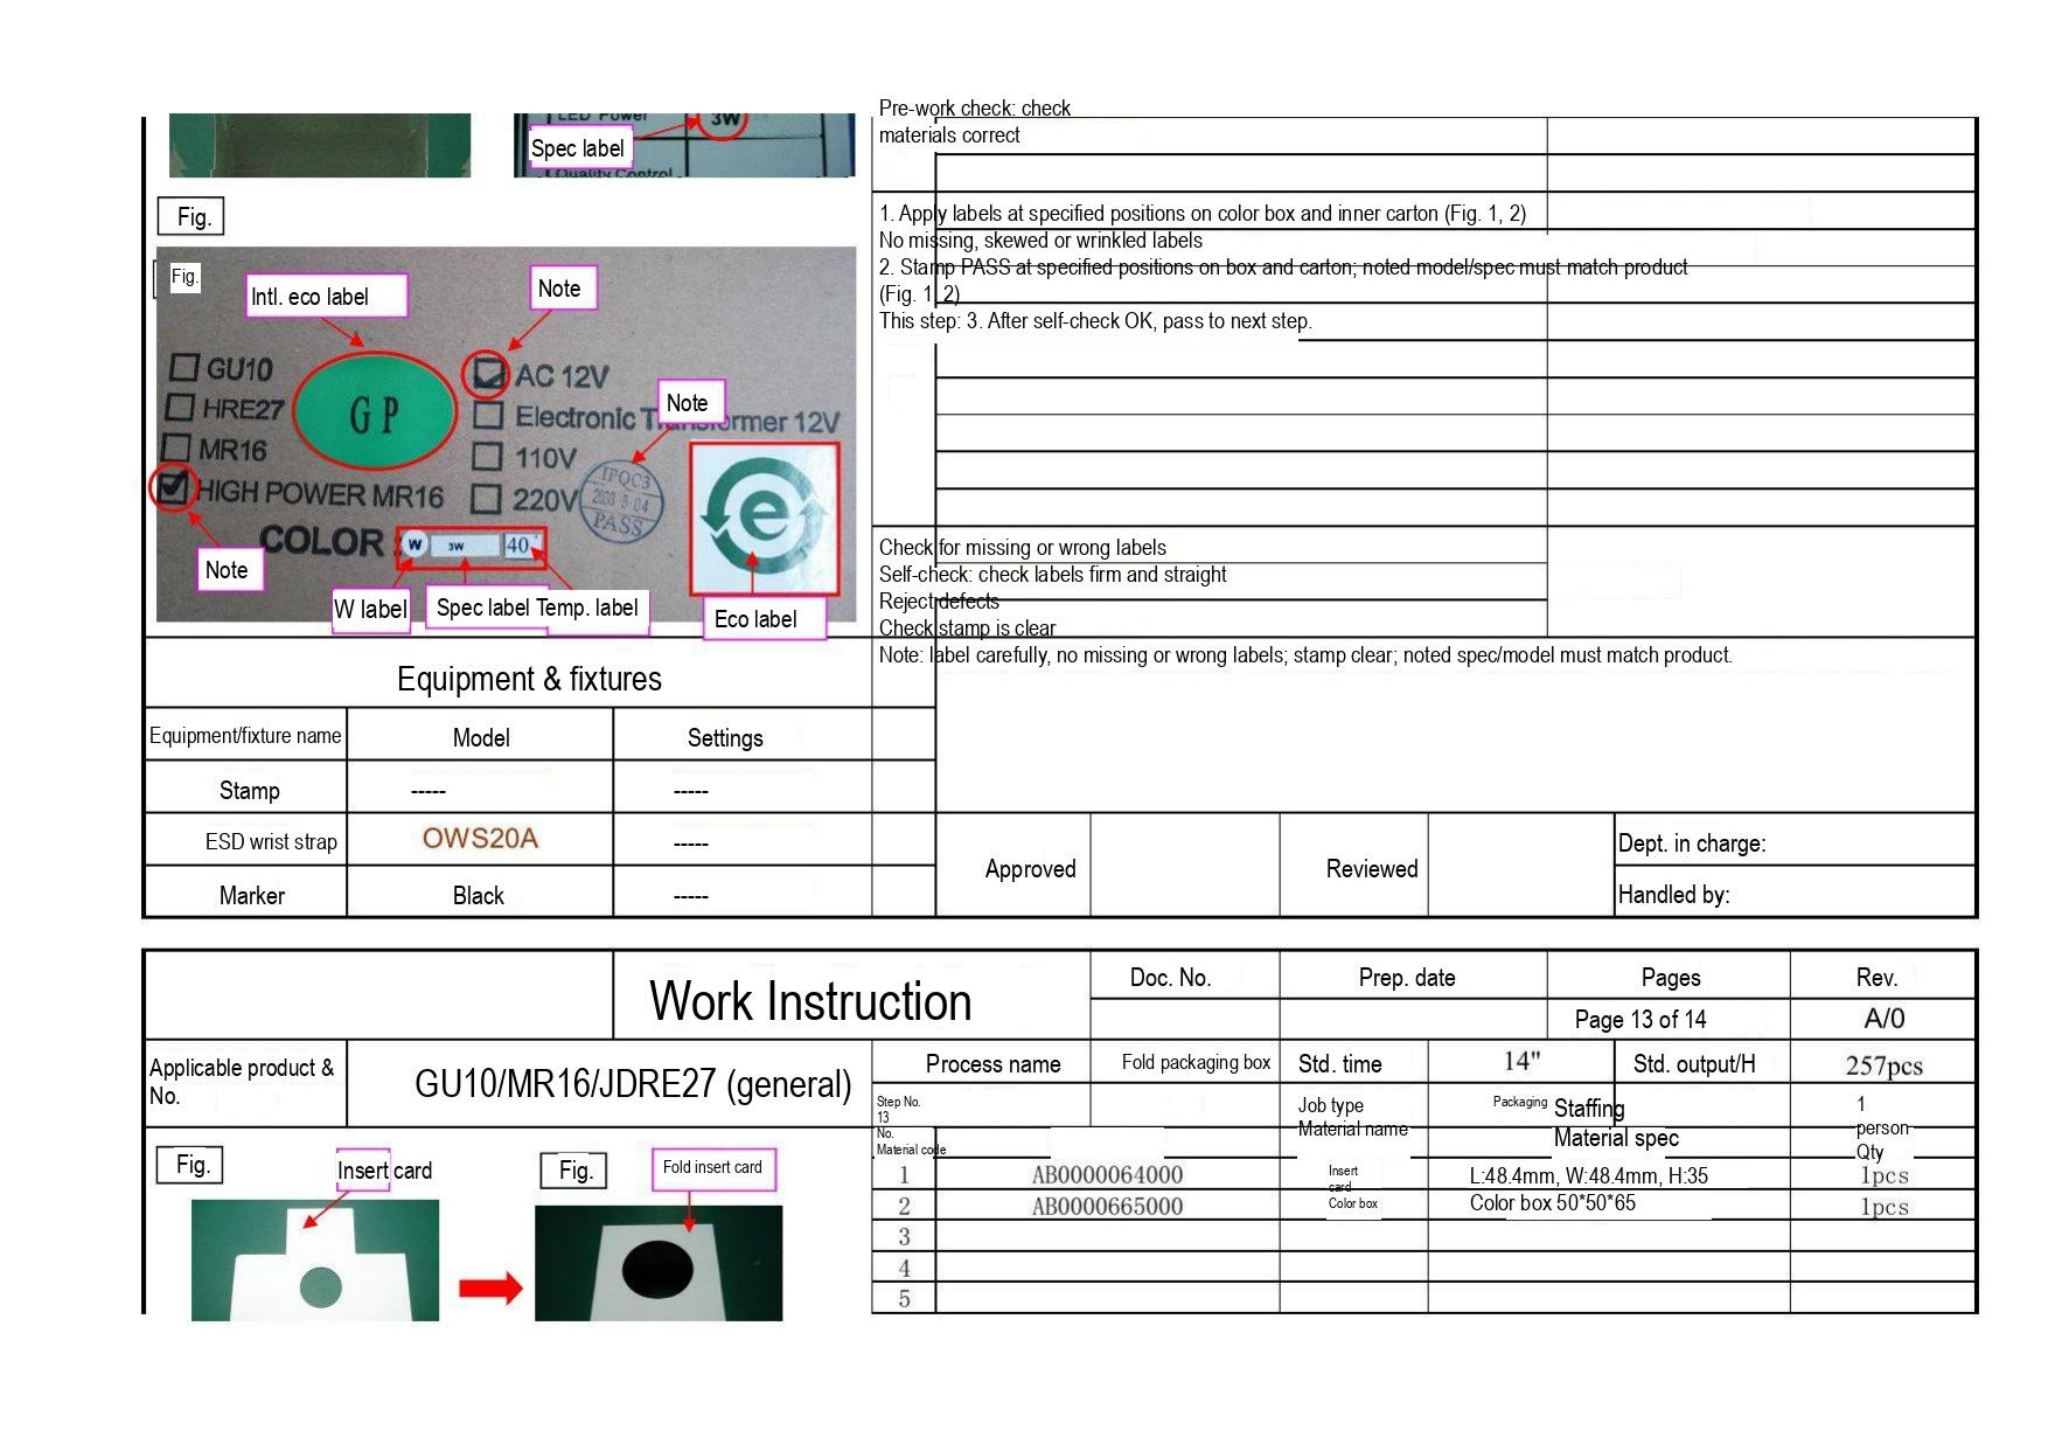LED Power

3W

Spec label

Quality Control

Fig.

Fig.

Intl. eco label

Note

GU10

HRE27

MR16

HIGH POWER MR16

G P

AC 12V

Electronic T Note rmer 12V

110V

220V

IPQC3
PASS

COLOR

W

3W

40

e

Note

W label

Spec label

Temp. label

Eco label

Pre-work check: check materials correct

1. Apply labels at specified positions on color box and inner carton (Fig. 1, 2)
No missing, skewed or wrinkled labels
2. Stamp PASS at specified positions on box and carton; noted model/spec must match product (Fig. 1, 2)
This step: 3. After self-check OK, pass to next step.

Check for missing or wrong labels
Self-check: check labels firm and straight
Reject defects
Check stamp is clear

Note: label carefully, no missing or wrong labels; stamp clear; noted spec/model must match product.

Equipment & fixtures

| Equipment/fixture name | Model | Settings |
|---|---|---|
| Stamp | ----- | ----- |
| ESD wrist strap | OWS20A | ----- |
| Marker | Black | ----- |

| Approved | | Reviewed | | Dept. in charge: |
|---|---|---|---|---|
| | | | | Handled by: |

| | Work Instruction | Doc. No. | Prep. date | Pages | Rev. |
|---|---|---|---|---|---|
| | | | | Page 13 of 14 | A/0 |

| Applicable product & No. | GU10/MR16/JDRE27 (general) |
|---|---|

| Process name | Fold packaging box | Std. time | 14" | Std. output/H | 257pcs |
|---|---|---|---|---|---|
| Step No. 13 | | Job type | Packaging | Staffing | 1 person |

| No. | Material code | Material name | Material spec | Qty |
|---|---|---|---|---|
| 1 | AB0000064000 | Insert card | L:48.4mm, W:48.4mm, H:35 | 1pcs |
| 2 | AB0000665000 | Color box | Color box 50*50*65 | 1pcs |
| 3 | | | | |
| 4 | | | | |
| 5 | | | | |

Fig.

Insert card

Fig.

Fold insert card
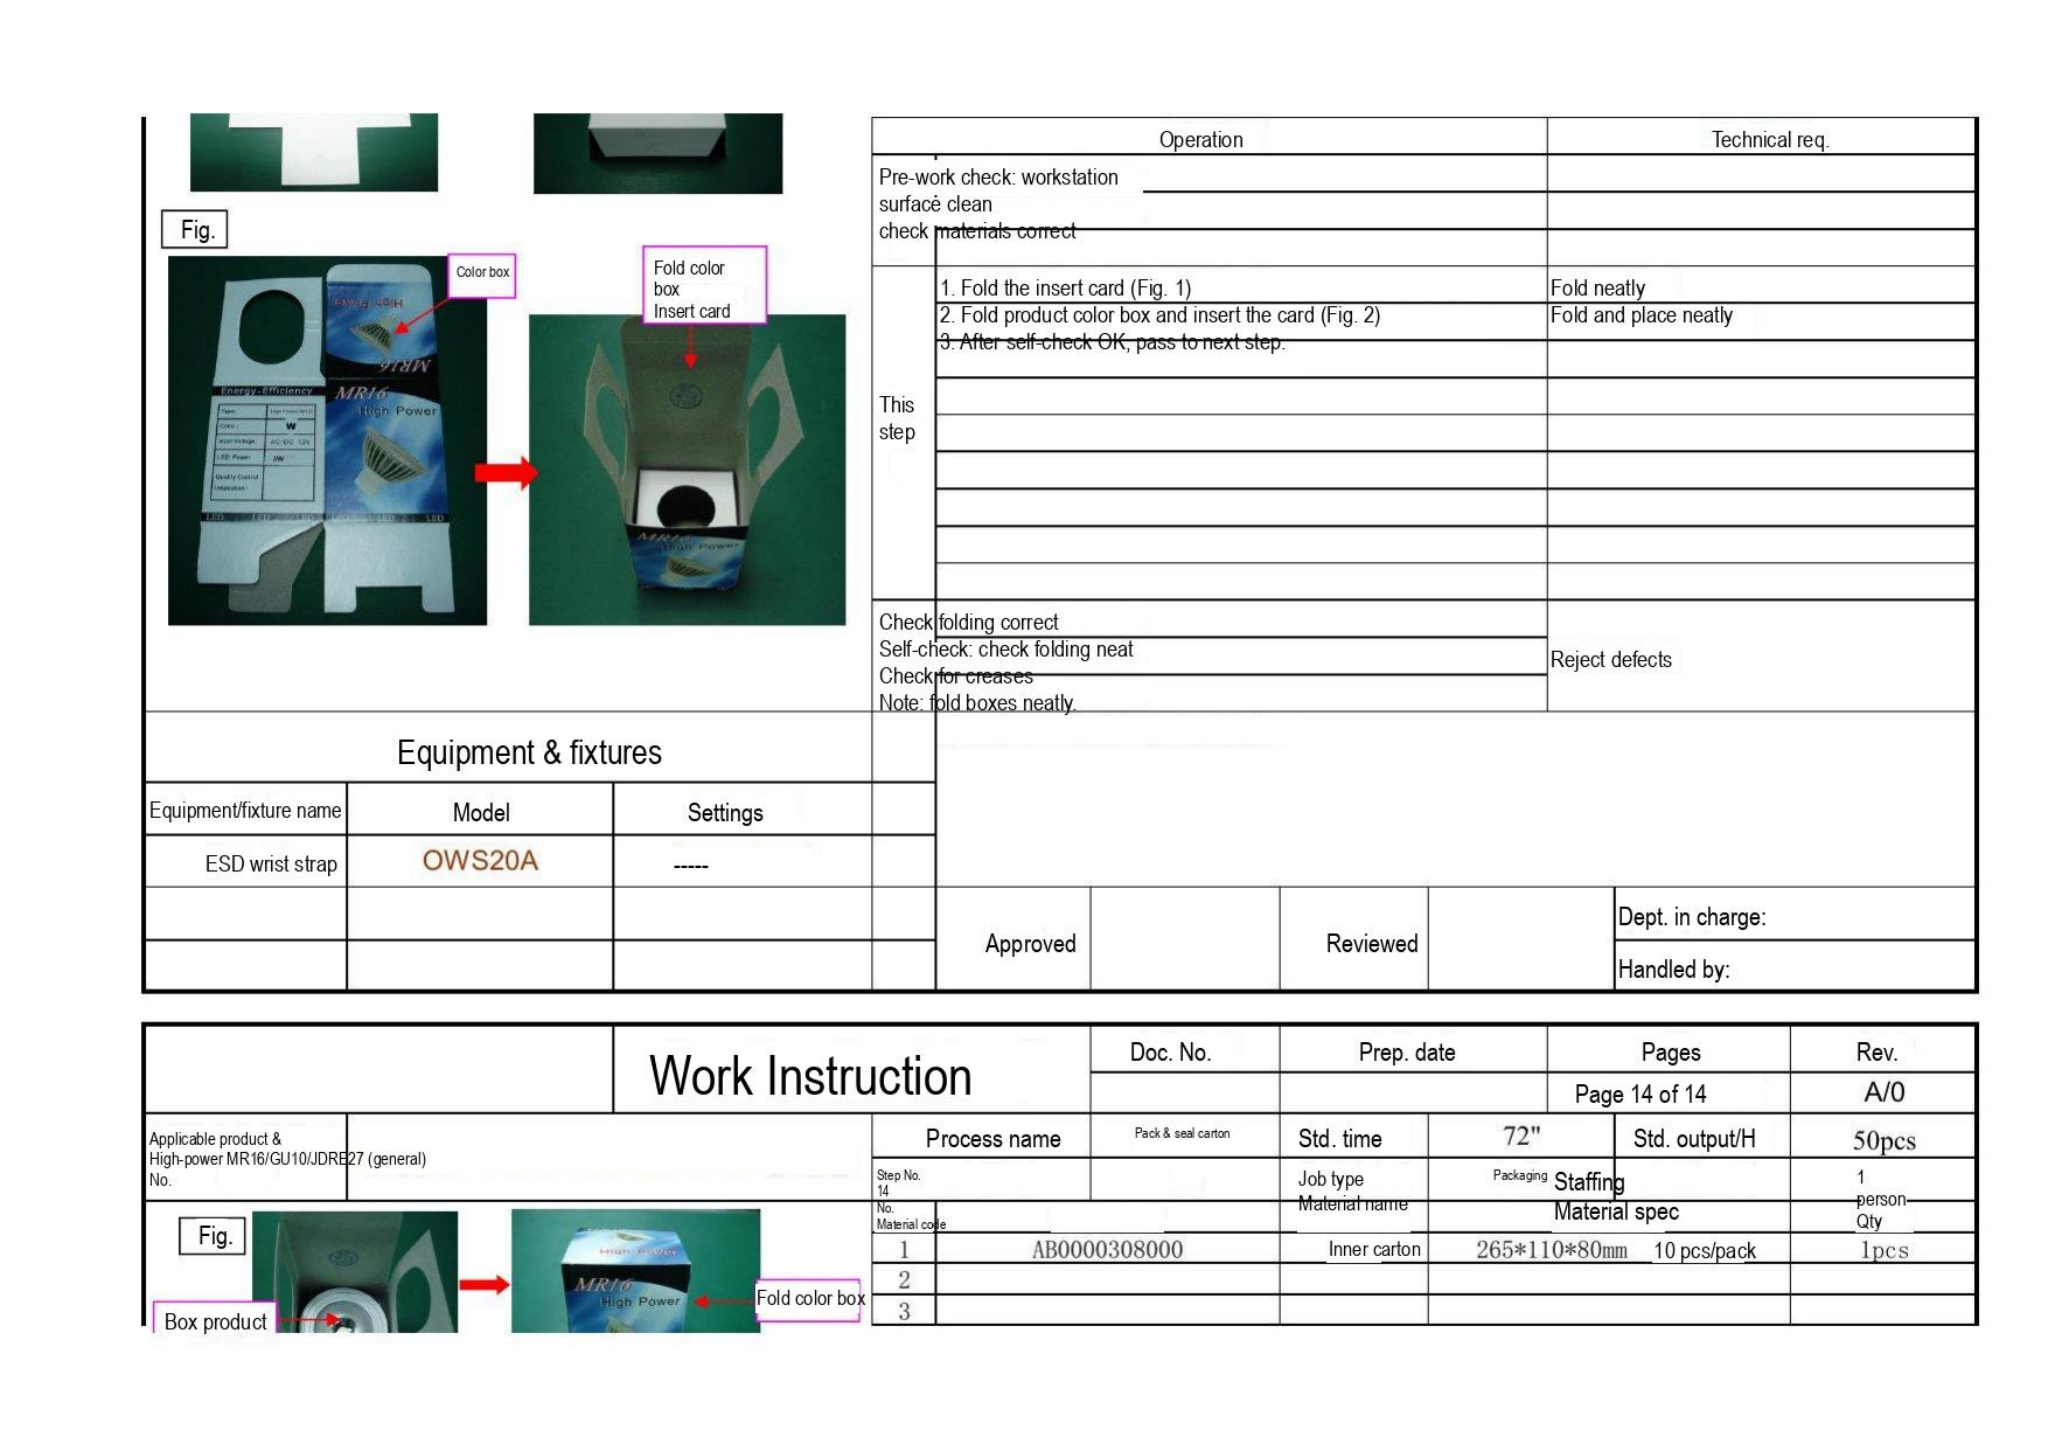Fig.

Color box

High Power
MR16
MR16
High Power
Energy-Efficiency

Fold color box
Insert card

| Operation | | Technical req. |
|---|---|---|
| Pre-work check: workstation surface clean<br>check materials correct | | |
| This step | 1. Fold the insert card (Fig. 1) | Fold neatly |
| | 2. Fold product color box and insert the card (Fig. 2) | Fold and place neatly |
| | 3. After self-check OK, pass to next step. | |
| Check folding correct<br>Self-check: check folding neat<br>Check for creases<br>Note: fold boxes neatly. | | Reject defects |

Equipment & fixtures

| Equipment/fixture name | Model | Settings |
|---|---|---|
| ESD wrist strap | OWS20A | ----- |
| | | |
| | | |

| Approved | | Reviewed | | Dept. in charge: |
|---|---|---|---|---|
| | | | | Handled by: |

| | Work Instruction | Doc. No. | Prep. date | Pages | Rev. |
|---|---|---|---|---|---|
| | | | | Page 14 of 14 | A/0 |

| Applicable product & High-power MR16/GU10/JDRE27 (general) No. | Process name | Pack & seal carton | Std. time | 72" | Std. output/H | 50pcs |
|---|---|---|---|---|---|---|
| | Step No. 14 | | Job type | Packaging | Staffing | 1 person |
| | No. Material code | | Material name | | Material spec | Qty |
| | 1 | AB0000308000 | Inner carton | 265*110*80mm | 10 pcs/pack | 1pcs |
| | 2 | | | | | |
| | 3 | | | | | |

Fig.

Box product

High Power
MR16
High Power

Fold color box
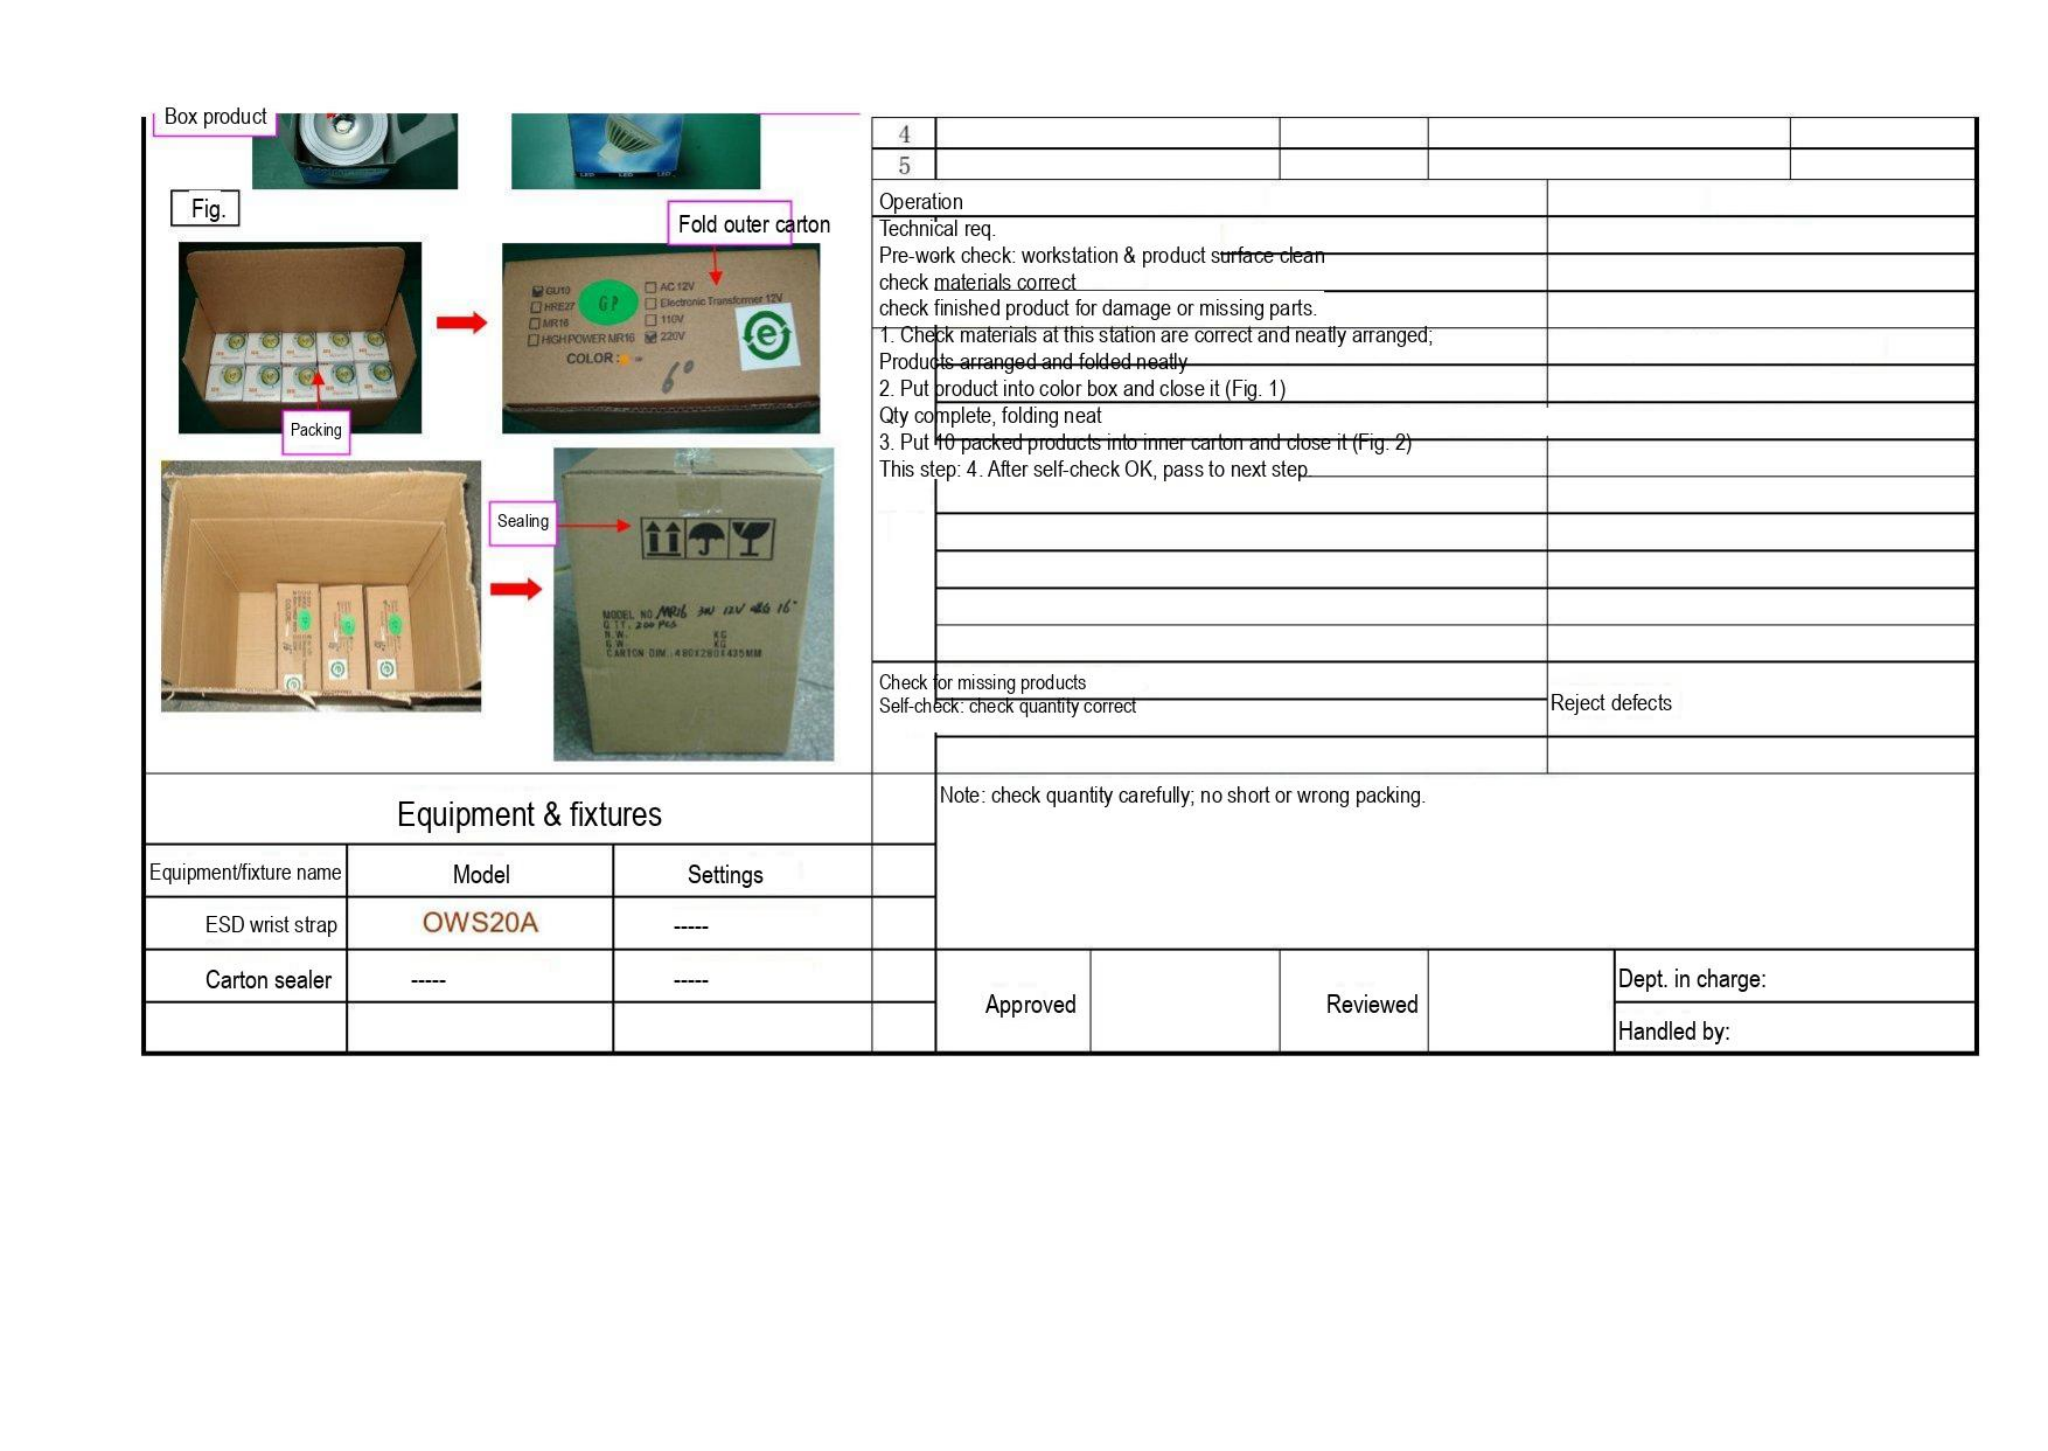Box product

Fig.

Fold outer carton

GU10
HRE27
MR16
HIGH POWER MR16
COLOR
AC 12V
Electronic Transformer 12V
110V
220V

Packing

Sealing

MODEL NO MR16 3W 12V
Q.TY. 200 PCS
N.W. KG
G.W. KG
CARTON DIM. 480X280X435MM

| 4 | | | | |
|---|---|---|---|---|
| 5 | | | | |

Operation
Technical req.
Pre-work check: workstation & product surface clean
check materials correct
check finished product for damage or missing parts.
1. Check materials at this station are correct and neatly arranged;
Products arranged and folded neatly
2. Put product into color box and close it (Fig. 1)
Qty complete, folding neat
3. Put 10 packed products into inner carton and close it (Fig. 2)
This step: 4. After self-check OK, pass to next step

Check for missing products
Self-check: check quantity correct

Reject defects

Note: check quantity carefully; no short or wrong packing.

Equipment & fixtures

| Equipment/fixture name | Model | Settings |
|---|---|---|
| ESD wrist strap | OWS20A | ----- |
| Carton sealer | ----- | ----- |
| | | |

| Approved | | Reviewed | | Dept. in charge: |
|---|---|---|---|---|
| | | | | Handled by: |